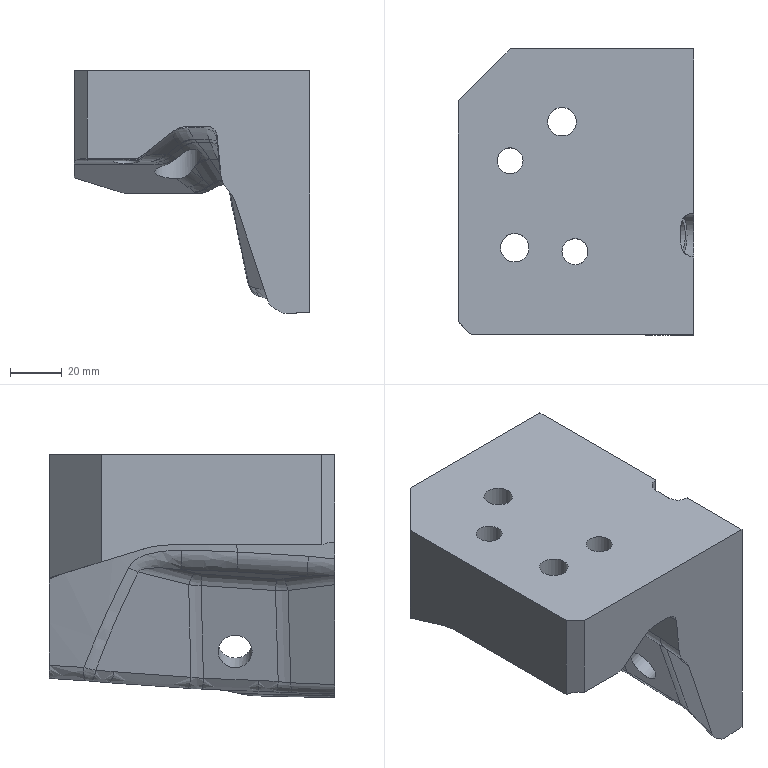Part | NX | features solid 2 | 1 solid | 115 faces | box 90.782 x 110 x 93.527 mm | volume 451093 mm3 | spline 53 | cylinder 37 | plane 24 | cone 1 | commonest cylinder face diameters 10 x6 16 x3 11 x2 20 x2 40 x2 340 x2